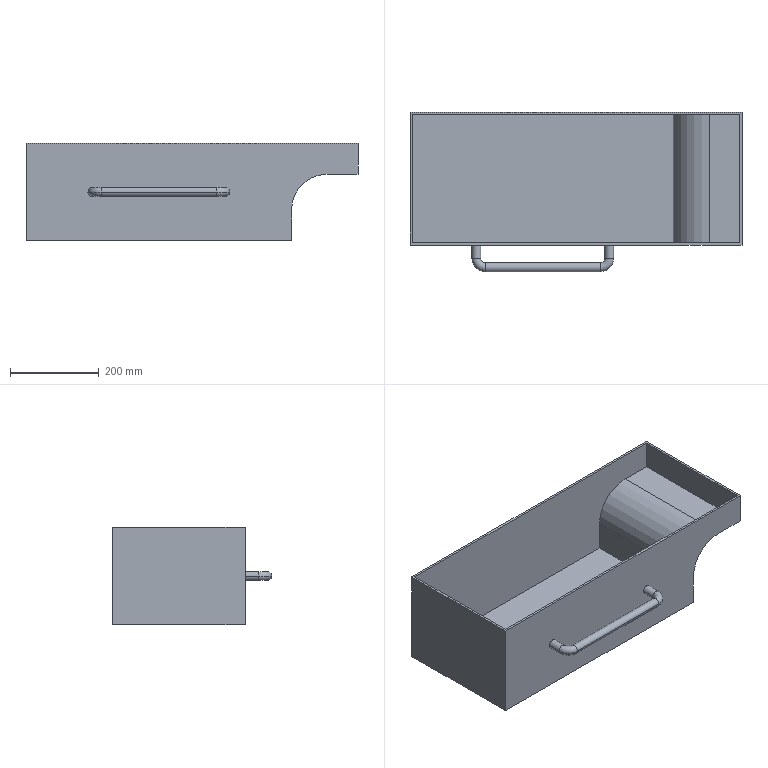Part | STEP file | Sugarcane segment collection box | 1 solid | 27 faces | box 750 x 360 x 220 mm | volume 3249841 mm3 | plane 15 | cylinder 8 | torus 4 | commonest cylinder face diameters 20 x6 160 x1 164 x1
STEP:
#1=CARTESIAN_POINT('',(-130.,-190.,0.));
#2=VERTEX_POINT('',#1);
#3=CARTESIAN_POINT('',(-130.,-210.,0.));
#4=VERTEX_POINT('',#3);
#5=CARTESIAN_POINT('',(-130.,-200.,0.));
#6=DIRECTION('',(-1.,0.,0.));
#7=DIRECTION('',(0.,0.,-1.));
#8=AXIS2_PLACEMENT_3D('',#5,#6,#7);
#9=CIRCLE('',#8,10.);
#10=EDGE_CURVE('',#2,#4,#9,.T.);
#11=ORIENTED_EDGE('',*,*,#10,.T.);
#12=CARTESIAN_POINT('',(-160.,-180.,0.));
#13=VERTEX_POINT('',#12);
#14=CARTESIAN_POINT('',(-130.,-180.,0.));
#15=DIRECTION('',(0.,0.,-1.));
#16=DIRECTION('',(-1.,0.,0.));
#17=AXIS2_PLACEMENT_3D('',#14,#15,#16);
#18=CIRCLE('',#17,30.);
#19=EDGE_CURVE('',#4,#13,#18,.T.);
#20=ORIENTED_EDGE('',*,*,#19,.T.);
#21=CARTESIAN_POINT('',(-140.,-180.,0.));
#22=VERTEX_POINT('',#21);
#23=CARTESIAN_POINT('',(-150.,-180.,0.));
#24=DIRECTION('',(0.,1.,0.));
#25=DIRECTION('',(0.,0.,-1.));
#26=AXIS2_PLACEMENT_3D('',#23,#24,#25);
#27=CIRCLE('',#26,10.);
#28=EDGE_CURVE('',#22,#13,#27,.T.);
#29=ORIENTED_EDGE('',*,*,#28,.F.);
#30=CARTESIAN_POINT('',(-130.,-180.,0.));
#31=DIRECTION('',(0.,0.,-1.));
#32=DIRECTION('',(-1.,0.,0.));
#33=AXIS2_PLACEMENT_3D('',#30,#31,#32);
#34=CIRCLE('',#33,10.);
#35=EDGE_CURVE('',#2,#22,#34,.T.);
#36=ORIENTED_EDGE('',*,*,#35,.F.);
#37=EDGE_LOOP('',(#11,#20,#29,#36));
#38=FACE_OUTER_BOUND('',#37,.T.);
#39=CARTESIAN_POINT('',(-130.,-180.,0.));
#40=DIRECTION('',(0.,0.,-1.));
#41=DIRECTION('',(-1.,0.,0.));
#42=AXIS2_PLACEMENT_3D('',#39,#40,#41);
#43=TOROIDAL_SURFACE('',#42,20.,10.);
#44=ADVANCED_FACE('',(#38),#43,.T.);
#45=CARTESIAN_POINT('',(140.,-180.,0.));
#46=VERTEX_POINT('',#45);
#47=CARTESIAN_POINT('',(160.,-180.,0.));
#48=VERTEX_POINT('',#47);
#49=CARTESIAN_POINT('',(150.,-180.,0.));
#50=DIRECTION('',(0.,-1.,0.));
#51=DIRECTION('',(0.,0.,-1.));
#52=AXIS2_PLACEMENT_3D('',#49,#50,#51);
#53=CIRCLE('',#52,10.);
#54=EDGE_CURVE('',#46,#48,#53,.T.);
#55=ORIENTED_EDGE('',*,*,#54,.T.);
#56=CARTESIAN_POINT('',(130.,-210.,0.));
#57=VERTEX_POINT('',#56);
#58=CARTESIAN_POINT('',(130.,-180.,0.));
#59=DIRECTION('',(0.,0.,-1.));
#60=DIRECTION('',(-1.,0.,0.));
#61=AXIS2_PLACEMENT_3D('',#58,#59,#60);
#62=CIRCLE('',#61,30.);
#63=EDGE_CURVE('',#48,#57,#62,.T.);
#64=ORIENTED_EDGE('',*,*,#63,.T.);
#65=CARTESIAN_POINT('',(130.,-190.,0.));
#66=VERTEX_POINT('',#65);
#67=CARTESIAN_POINT('',(130.,-200.,0.));
#68=DIRECTION('',(-1.,0.,0.));
#69=DIRECTION('',(0.,0.,-1.));
#70=AXIS2_PLACEMENT_3D('',#67,#68,#69);
#71=CIRCLE('',#70,10.);
#72=EDGE_CURVE('',#66,#57,#71,.T.);
#73=ORIENTED_EDGE('',*,*,#72,.F.);
#74=CARTESIAN_POINT('',(130.,-180.,0.));
#75=DIRECTION('',(0.,0.,-1.));
#76=DIRECTION('',(-1.,0.,0.));
#77=AXIS2_PLACEMENT_3D('',#74,#75,#76);
#78=CIRCLE('',#77,10.);
#79=EDGE_CURVE('',#46,#66,#78,.T.);
#80=ORIENTED_EDGE('',*,*,#79,.F.);
#81=EDGE_LOOP('',(#55,#64,#73,#80));
#82=FACE_OUTER_BOUND('',#81,.T.);
#83=CARTESIAN_POINT('',(130.,-180.,0.));
#84=DIRECTION('',(0.,0.,-1.));
#85=DIRECTION('',(-1.,0.,0.));
#86=AXIS2_PLACEMENT_3D('',#83,#84,#85);
#87=TOROIDAL_SURFACE('',#86,20.,10.);
#88=ADVANCED_FACE('',(#82),#87,.T.);
#89=CARTESIAN_POINT('',(-150.,-180.,0.));
#90=DIRECTION('',(0.,1.,0.));
#91=DIRECTION('',(0.,0.,-1.));
#92=AXIS2_PLACEMENT_3D('',#89,#90,#91);
#93=CIRCLE('',#92,10.);
#94=EDGE_CURVE('',#13,#22,#93,.T.);
#95=ORIENTED_EDGE('',*,*,#94,.T.);
#96=CARTESIAN_POINT('',(-140.,-150.,0.));
#97=VERTEX_POINT('',#96);
#98=CARTESIAN_POINT('',(-140.,-180.,0.));
#99=DIRECTION('',(0.,1.,0.));
#100=VECTOR('',#99,1000.);
#101=LINE('',#98,#100);
#102=EDGE_CURVE('',#22,#97,#101,.T.);
#103=ORIENTED_EDGE('',*,*,#102,.T.);
#104=CARTESIAN_POINT('',(-160.,-150.,0.));
#105=VERTEX_POINT('',#104);
#106=CARTESIAN_POINT('',(-150.,-150.,0.));
#107=DIRECTION('',(0.,1.,0.));
#108=DIRECTION('',(0.,0.,-1.));
#109=AXIS2_PLACEMENT_3D('',#106,#107,#108);
#110=CIRCLE('',#109,10.);
#111=EDGE_CURVE('',#105,#97,#110,.T.);
#112=ORIENTED_EDGE('',*,*,#111,.F.);
#113=CARTESIAN_POINT('',(-160.,-180.,0.));
#114=DIRECTION('',(0.,1.,0.));
#115=VECTOR('',#114,1000.);
#116=LINE('',#113,#115);
#117=EDGE_CURVE('',#13,#105,#116,.T.);
#118=ORIENTED_EDGE('',*,*,#117,.F.);
#119=EDGE_LOOP('',(#95,#103,#112,#118));
#120=FACE_OUTER_BOUND('',#119,.T.);
#121=CARTESIAN_POINT('',(-150.,-180.,0.));
#122=DIRECTION('',(0.,1.,0.));
#123=DIRECTION('',(-1.,0.,0.));
#124=AXIS2_PLACEMENT_3D('',#121,#122,#123);
#125=CYLINDRICAL_SURFACE('',#124,10.);
#126=ADVANCED_FACE('',(#120),#125,.T.);
#127=CARTESIAN_POINT('',(130.,-200.,0.));
#128=DIRECTION('',(-1.,0.,0.));
#129=DIRECTION('',(0.,0.,-1.));
#130=AXIS2_PLACEMENT_3D('',#127,#128,#129);
#131=CIRCLE('',#130,10.);
#132=EDGE_CURVE('',#57,#66,#131,.T.);
#133=ORIENTED_EDGE('',*,*,#132,.T.);
#134=CARTESIAN_POINT('',(130.,-190.,0.));
#135=DIRECTION('',(-1.,0.,0.));
#136=VECTOR('',#135,1000.);
#137=LINE('',#134,#136);
#138=EDGE_CURVE('',#66,#2,#137,.T.);
#139=ORIENTED_EDGE('',*,*,#138,.T.);
#140=CARTESIAN_POINT('',(-130.,-200.,0.));
#141=DIRECTION('',(-1.,0.,0.));
#142=DIRECTION('',(0.,0.,-1.));
#143=AXIS2_PLACEMENT_3D('',#140,#141,#142);
#144=CIRCLE('',#143,10.);
#145=EDGE_CURVE('',#4,#2,#144,.T.);
#146=ORIENTED_EDGE('',*,*,#145,.F.);
#147=CARTESIAN_POINT('',(130.,-210.,0.));
#148=DIRECTION('',(-1.,0.,0.));
#149=VECTOR('',#148,1000.);
#150=LINE('',#147,#149);
#151=EDGE_CURVE('',#57,#4,#150,.T.);
#152=ORIENTED_EDGE('',*,*,#151,.F.);
#153=EDGE_LOOP('',(#133,#139,#146,#152));
#154=FACE_OUTER_BOUND('',#153,.T.);
#155=CARTESIAN_POINT('',(130.,-200.,0.));
#156=DIRECTION('',(-1.,0.,0.));
#157=DIRECTION('',(0.,-1.,0.));
#158=AXIS2_PLACEMENT_3D('',#155,#156,#157);
#159=CYLINDRICAL_SURFACE('',#158,10.);
#160=ADVANCED_FACE('',(#154),#159,.T.);
#161=CARTESIAN_POINT('',(160.,-150.,0.));
#162=VERTEX_POINT('',#161);
#163=CARTESIAN_POINT('',(140.,-150.,0.));
#164=VERTEX_POINT('',#163);
#165=CARTESIAN_POINT('',(150.,-150.,0.));
#166=DIRECTION('',(0.,-1.,0.));
#167=DIRECTION('',(0.,0.,-1.));
#168=AXIS2_PLACEMENT_3D('',#165,#166,#167);
#169=CIRCLE('',#168,10.);
#170=EDGE_CURVE('',#162,#164,#169,.T.);
#171=ORIENTED_EDGE('',*,*,#170,.T.);
#172=CARTESIAN_POINT('',(140.,-150.,0.));
#173=DIRECTION('',(0.,-1.,0.));
#174=VECTOR('',#173,1000.);
#175=LINE('',#172,#174);
#176=EDGE_CURVE('',#164,#46,#175,.T.);
#177=ORIENTED_EDGE('',*,*,#176,.T.);
#178=CARTESIAN_POINT('',(150.,-180.,0.));
#179=DIRECTION('',(0.,-1.,0.));
#180=DIRECTION('',(0.,0.,-1.));
#181=AXIS2_PLACEMENT_3D('',#178,#179,#180);
#182=CIRCLE('',#181,10.);
#183=EDGE_CURVE('',#48,#46,#182,.T.);
#184=ORIENTED_EDGE('',*,*,#183,.F.);
#185=CARTESIAN_POINT('',(160.,-150.,0.));
#186=DIRECTION('',(0.,-1.,0.));
#187=VECTOR('',#186,1000.);
#188=LINE('',#185,#187);
#189=EDGE_CURVE('',#162,#48,#188,.T.);
#190=ORIENTED_EDGE('',*,*,#189,.F.);
#191=EDGE_LOOP('',(#171,#177,#184,#190));
#192=FACE_OUTER_BOUND('',#191,.T.);
#193=CARTESIAN_POINT('',(150.,-150.,0.));
#194=DIRECTION('',(0.,-1.,0.));
#195=DIRECTION('',(1.,0.,0.));
#196=AXIS2_PLACEMENT_3D('',#193,#194,#195);
#197=CYLINDRICAL_SURFACE('',#196,10.);
#198=ADVANCED_FACE('',(#192),#197,.T.);
#199=CARTESIAN_POINT('',(445.,145.,110.));
#200=VERTEX_POINT('',#199);
#201=CARTESIAN_POINT('',(445.,-145.,110.));
#202=VERTEX_POINT('',#201);
#203=CARTESIAN_POINT('',(445.,0.,110.));
#204=DIRECTION('',(0.,-1.,0.));
#205=VECTOR('',#204,1000.);
#206=LINE('',#203,#205);
#207=EDGE_CURVE('',#200,#202,#206,.T.);
#208=ORIENTED_EDGE('',*,*,#207,.T.);
#209=CARTESIAN_POINT('',(-295.,-145.,110.));
#210=VERTEX_POINT('',#209);
#211=CARTESIAN_POINT('',(-300.,-145.,110.));
#212=DIRECTION('',(1.,0.,0.));
#213=VECTOR('',#212,1000.);
#214=LINE('',#211,#213);
#215=EDGE_CURVE('',#210,#202,#214,.T.);
#216=ORIENTED_EDGE('',*,*,#215,.F.);
#217=CARTESIAN_POINT('',(-295.,145.,110.));
#218=VERTEX_POINT('',#217);
#219=CARTESIAN_POINT('',(-295.,150.,110.));
#220=DIRECTION('',(0.,-1.,0.));
#221=VECTOR('',#220,1000.);
#222=LINE('',#219,#221);
#223=EDGE_CURVE('',#218,#210,#222,.T.);
#224=ORIENTED_EDGE('',*,*,#223,.F.);
#225=CARTESIAN_POINT('',(-300.,145.,110.));
#226=DIRECTION('',(-1.,0.,0.));
#227=VECTOR('',#226,1000.);
#228=LINE('',#225,#227);
#229=EDGE_CURVE('',#200,#218,#228,.T.);
#230=ORIENTED_EDGE('',*,*,#229,.F.);
#231=EDGE_LOOP('',(#208,#216,#224,#230));
#232=FACE_BOUND('',#231,.T.);
#233=CARTESIAN_POINT('',(-300.,-150.,110.));
#234=VERTEX_POINT('',#233);
#235=CARTESIAN_POINT('',(450.,-150.,110.));
#236=VERTEX_POINT('',#235);
#237=CARTESIAN_POINT('',(-300.,-150.,110.));
#238=DIRECTION('',(1.,0.,0.));
#239=VECTOR('',#238,1000.);
#240=LINE('',#237,#239);
#241=EDGE_CURVE('',#234,#236,#240,.T.);
#242=ORIENTED_EDGE('',*,*,#241,.T.);
#243=CARTESIAN_POINT('',(450.,150.,110.));
#244=VERTEX_POINT('',#243);
#245=CARTESIAN_POINT('',(450.,-150.,110.));
#246=DIRECTION('',(0.,-1.,0.));
#247=VECTOR('',#246,1000.);
#248=LINE('',#245,#247);
#249=EDGE_CURVE('',#244,#236,#248,.T.);
#250=ORIENTED_EDGE('',*,*,#249,.F.);
#251=CARTESIAN_POINT('',(-300.,150.,110.));
#252=VERTEX_POINT('',#251);
#253=CARTESIAN_POINT('',(-300.,150.,110.));
#254=DIRECTION('',(-1.,0.,0.));
#255=VECTOR('',#254,1000.);
#256=LINE('',#253,#255);
#257=EDGE_CURVE('',#244,#252,#256,.T.);
#258=ORIENTED_EDGE('',*,*,#257,.T.);
#259=CARTESIAN_POINT('',(-300.,150.,110.));
#260=DIRECTION('',(0.,-1.,0.));
#261=VECTOR('',#260,1000.);
#262=LINE('',#259,#261);
#263=EDGE_CURVE('',#252,#234,#262,.T.);
#264=ORIENTED_EDGE('',*,*,#263,.T.);
#265=EDGE_LOOP('',(#242,#250,#258,#264));
#266=FACE_OUTER_BOUND('',#265,.T.);
#267=CARTESIAN_POINT('',(0.,0.,110.));
#268=DIRECTION('',(0.,0.,1.));
#269=DIRECTION('',(1.,0.,0.));
#270=AXIS2_PLACEMENT_3D('',#267,#268,#269);
#271=PLANE('',#270);
#272=ADVANCED_FACE('',(#232,#266),#271,.T.);
#273=CARTESIAN_POINT('',(300.,150.,-40.));
#274=VERTEX_POINT('',#273);
#275=CARTESIAN_POINT('',(300.,150.,-110.));
#276=VERTEX_POINT('',#275);
#277=CARTESIAN_POINT('',(300.,150.,110.));
#278=DIRECTION('',(0.,0.,-1.));
#279=VECTOR('',#278,1000.);
#280=LINE('',#277,#279);
#281=EDGE_CURVE('',#274,#276,#280,.T.);
#282=ORIENTED_EDGE('',*,*,#281,.F.);
#283=CARTESIAN_POINT('',(300.,-150.,-40.));
#284=VERTEX_POINT('',#283);
#285=CARTESIAN_POINT('',(300.,-150.,-40.));
#286=DIRECTION('',(0.,-1.,0.));
#287=VECTOR('',#286,1000.);
#288=LINE('',#285,#287);
#289=EDGE_CURVE('',#274,#284,#288,.T.);
#290=ORIENTED_EDGE('',*,*,#289,.T.);
#291=CARTESIAN_POINT('',(300.,-150.,-110.));
#292=VERTEX_POINT('',#291);
#293=CARTESIAN_POINT('',(300.,-150.,110.));
#294=DIRECTION('',(0.,0.,-1.));
#295=VECTOR('',#294,1000.);
#296=LINE('',#293,#295);
#297=EDGE_CURVE('',#284,#292,#296,.T.);
#298=ORIENTED_EDGE('',*,*,#297,.T.);
#299=CARTESIAN_POINT('',(300.,150.,-110.));
#300=DIRECTION('',(0.,1.,0.));
#301=VECTOR('',#300,1000.);
#302=LINE('',#299,#301);
#303=EDGE_CURVE('',#292,#276,#302,.T.);
#304=ORIENTED_EDGE('',*,*,#303,.T.);
#305=EDGE_LOOP('',(#282,#290,#298,#304));
#306=FACE_OUTER_BOUND('',#305,.T.);
#307=CARTESIAN_POINT('',(300.,150.,110.));
#308=DIRECTION('',(-1.,0.,0.));
#309=DIRECTION('',(0.,0.,1.));
#310=AXIS2_PLACEMENT_3D('',#307,#308,#309);
#311=PLANE('',#310);
#312=ADVANCED_FACE('',(#306),#311,.F.);
#313=ORIENTED_EDGE('',*,*,#170,.F.);
#314=CARTESIAN_POINT('',(150.,-150.,0.));
#315=DIRECTION('',(0.,-1.,0.));
#316=DIRECTION('',(0.,0.,-1.));
#317=AXIS2_PLACEMENT_3D('',#314,#315,#316);
#318=CIRCLE('',#317,10.);
#319=EDGE_CURVE('',#164,#162,#318,.T.);
#320=ORIENTED_EDGE('',*,*,#319,.F.);
#321=EDGE_LOOP('',(#313,#320));
#322=FACE_BOUND('',#321,.T.);
#323=CARTESIAN_POINT('',(-300.,-150.,-110.));
#324=VERTEX_POINT('',#323);
#325=CARTESIAN_POINT('',(-300.,-150.,-110.));
#326=DIRECTION('',(1.,0.,0.));
#327=VECTOR('',#326,1000.);
#328=LINE('',#325,#327);
#329=EDGE_CURVE('',#324,#292,#328,.T.);
#330=ORIENTED_EDGE('',*,*,#329,.T.);
#331=ORIENTED_EDGE('',*,*,#297,.F.);
#332=CARTESIAN_POINT('',(380.,-150.,40.));
#333=VERTEX_POINT('',#332);
#334=CARTESIAN_POINT('',(380.,-150.,-40.));
#335=DIRECTION('',(0.,1.,0.));
#336=DIRECTION('',(0.,0.,1.));
#337=AXIS2_PLACEMENT_3D('',#334,#335,#336);
#338=CIRCLE('',#337,80.);
#339=EDGE_CURVE('',#284,#333,#338,.T.);
#340=ORIENTED_EDGE('',*,*,#339,.T.);
#341=CARTESIAN_POINT('',(450.,-150.,40.));
#342=VERTEX_POINT('',#341);
#343=CARTESIAN_POINT('',(450.,-150.,40.));
#344=DIRECTION('',(-1.,0.,0.));
#345=VECTOR('',#344,1000.);
#346=LINE('',#343,#345);
#347=EDGE_CURVE('',#342,#333,#346,.T.);
#348=ORIENTED_EDGE('',*,*,#347,.F.);
#349=CARTESIAN_POINT('',(450.,-150.,110.));
#350=DIRECTION('',(0.,0.,-1.));
#351=VECTOR('',#350,1000.);
#352=LINE('',#349,#351);
#353=EDGE_CURVE('',#236,#342,#352,.T.);
#354=ORIENTED_EDGE('',*,*,#353,.F.);
#355=ORIENTED_EDGE('',*,*,#241,.F.);
#356=CARTESIAN_POINT('',(-300.,-150.,110.));
#357=DIRECTION('',(0.,0.,-1.));
#358=VECTOR('',#357,1000.);
#359=LINE('',#356,#358);
#360=EDGE_CURVE('',#234,#324,#359,.T.);
#361=ORIENTED_EDGE('',*,*,#360,.T.);
#362=EDGE_LOOP('',(#330,#331,#340,#348,#354,#355,#361));
#363=FACE_OUTER_BOUND('',#362,.T.);
#364=ORIENTED_EDGE('',*,*,#111,.T.);
#365=CARTESIAN_POINT('',(-150.,-150.,0.));
#366=DIRECTION('',(0.,1.,0.));
#367=DIRECTION('',(0.,0.,-1.));
#368=AXIS2_PLACEMENT_3D('',#365,#366,#367);
#369=CIRCLE('',#368,10.);
#370=EDGE_CURVE('',#97,#105,#369,.T.);
#371=ORIENTED_EDGE('',*,*,#370,.T.);
#372=EDGE_LOOP('',(#364,#371));
#373=FACE_BOUND('',#372,.T.);
#374=CARTESIAN_POINT('',(-300.,-150.,110.));
#375=DIRECTION('',(0.,1.,0.));
#376=DIRECTION('',(0.,0.,1.));
#377=AXIS2_PLACEMENT_3D('',#374,#375,#376);
#378=PLANE('',#377);
#379=ADVANCED_FACE('',(#322,#363,#373),#378,.F.);
#380=CARTESIAN_POINT('',(-300.,150.,-110.));
#381=VERTEX_POINT('',#380);
#382=CARTESIAN_POINT('',(-300.,150.,-110.));
#383=DIRECTION('',(-1.,0.,0.));
#384=VECTOR('',#383,1000.);
#385=LINE('',#382,#384);
#386=EDGE_CURVE('',#276,#381,#385,.T.);
#387=ORIENTED_EDGE('',*,*,#386,.T.);
#388=CARTESIAN_POINT('',(-300.,150.,110.));
#389=DIRECTION('',(0.,0.,-1.));
#390=VECTOR('',#389,1000.);
#391=LINE('',#388,#390);
#392=EDGE_CURVE('',#252,#381,#391,.T.);
#393=ORIENTED_EDGE('',*,*,#392,.F.);
#394=ORIENTED_EDGE('',*,*,#257,.F.);
#395=CARTESIAN_POINT('',(450.,150.,40.));
#396=VERTEX_POINT('',#395);
#397=CARTESIAN_POINT('',(450.,150.,110.));
#398=DIRECTION('',(0.,0.,1.));
#399=VECTOR('',#398,1000.);
#400=LINE('',#397,#399);
#401=EDGE_CURVE('',#396,#244,#400,.T.);
#402=ORIENTED_EDGE('',*,*,#401,.F.);
#403=CARTESIAN_POINT('',(380.,150.,40.));
#404=VERTEX_POINT('',#403);
#405=CARTESIAN_POINT('',(450.,150.,40.));
#406=DIRECTION('',(-1.,0.,0.));
#407=VECTOR('',#406,1000.);
#408=LINE('',#405,#407);
#409=EDGE_CURVE('',#396,#404,#408,.T.);
#410=ORIENTED_EDGE('',*,*,#409,.T.);
#411=CARTESIAN_POINT('',(380.,150.,-40.));
#412=DIRECTION('',(0.,-1.,0.));
#413=DIRECTION('',(0.,0.,-1.));
#414=AXIS2_PLACEMENT_3D('',#411,#412,#413);
#415=CIRCLE('',#414,80.);
#416=EDGE_CURVE('',#404,#274,#415,.T.);
#417=ORIENTED_EDGE('',*,*,#416,.T.);
#418=ORIENTED_EDGE('',*,*,#281,.T.);
#419=EDGE_LOOP('',(#387,#393,#394,#402,#410,#417,#418));
#420=FACE_OUTER_BOUND('',#419,.T.);
#421=CARTESIAN_POINT('',(-300.,150.,110.));
#422=DIRECTION('',(0.,-1.,0.));
#423=DIRECTION('',(0.,0.,-1.));
#424=AXIS2_PLACEMENT_3D('',#421,#422,#423);
#425=PLANE('',#424);
#426=ADVANCED_FACE('',(#420),#425,.F.);
#427=CARTESIAN_POINT('',(-300.,150.,-110.));
#428=DIRECTION('',(0.,-1.,0.));
#429=VECTOR('',#428,1000.);
#430=LINE('',#427,#429);
#431=EDGE_CURVE('',#381,#324,#430,.T.);
#432=ORIENTED_EDGE('',*,*,#431,.T.);
#433=ORIENTED_EDGE('',*,*,#360,.F.);
#434=ORIENTED_EDGE('',*,*,#263,.F.);
#435=ORIENTED_EDGE('',*,*,#392,.T.);
#436=EDGE_LOOP('',(#432,#433,#434,#435));
#437=FACE_OUTER_BOUND('',#436,.T.);
#438=CARTESIAN_POINT('',(-300.,150.,110.));
#439=DIRECTION('',(1.,0.,0.));
#440=DIRECTION('',(0.,0.,-1.));
#441=AXIS2_PLACEMENT_3D('',#438,#439,#440);
#442=PLANE('',#441);
#443=ADVANCED_FACE('',(#437),#442,.F.);
#444=ORIENTED_EDGE('',*,*,#303,.F.);
#445=ORIENTED_EDGE('',*,*,#329,.F.);
#446=ORIENTED_EDGE('',*,*,#431,.F.);
#447=ORIENTED_EDGE('',*,*,#386,.F.);
#448=EDGE_LOOP('',(#444,#445,#446,#447));
#449=FACE_OUTER_BOUND('',#448,.T.);
#450=CARTESIAN_POINT('',(0.,0.,-110.));
#451=DIRECTION('',(0.,0.,1.));
#452=DIRECTION('',(1.,0.,0.));
#453=AXIS2_PLACEMENT_3D('',#450,#451,#452);
#454=PLANE('',#453);
#455=ADVANCED_FACE('',(#449),#454,.F.);
#456=CARTESIAN_POINT('',(295.,-145.,-37.));
#457=VERTEX_POINT('',#456);
#458=CARTESIAN_POINT('',(295.,-145.,-105.));
#459=VERTEX_POINT('',#458);
#460=CARTESIAN_POINT('',(295.,-145.,110.));
#461=DIRECTION('',(0.,0.,-1.));
#462=VECTOR('',#461,1000.);
#463=LINE('',#460,#462);
#464=EDGE_CURVE('',#457,#459,#463,.T.);
#465=ORIENTED_EDGE('',*,*,#464,.F.);
#466=CARTESIAN_POINT('',(295.,145.,-37.));
#467=VERTEX_POINT('',#466);
#468=CARTESIAN_POINT('',(295.,150.,-37.));
#469=DIRECTION('',(0.,1.,0.));
#470=VECTOR('',#469,1000.);
#471=LINE('',#468,#470);
#472=EDGE_CURVE('',#457,#467,#471,.T.);
#473=ORIENTED_EDGE('',*,*,#472,.T.);
#474=CARTESIAN_POINT('',(295.,145.,-105.));
#475=VERTEX_POINT('',#474);
#476=CARTESIAN_POINT('',(295.,145.,110.));
#477=DIRECTION('',(0.,0.,-1.));
#478=VECTOR('',#477,1000.);
#479=LINE('',#476,#478);
#480=EDGE_CURVE('',#467,#475,#479,.T.);
#481=ORIENTED_EDGE('',*,*,#480,.T.);
#482=CARTESIAN_POINT('',(295.,150.,-105.));
#483=DIRECTION('',(0.,1.,0.));
#484=VECTOR('',#483,1000.);
#485=LINE('',#482,#484);
#486=EDGE_CURVE('',#459,#475,#485,.T.);
#487=ORIENTED_EDGE('',*,*,#486,.F.);
#488=EDGE_LOOP('',(#465,#473,#481,#487));
#489=FACE_OUTER_BOUND('',#488,.T.);
#490=CARTESIAN_POINT('',(295.,150.,110.));
#491=DIRECTION('',(-1.,0.,0.));
#492=DIRECTION('',(0.,0.,1.));
#493=AXIS2_PLACEMENT_3D('',#490,#491,#492);
#494=PLANE('',#493);
#495=ADVANCED_FACE('',(#489),#494,.T.);
#496=ORIENTED_EDGE('',*,*,#480,.F.);
#497=CARTESIAN_POINT('',(377.,145.,45.));
#498=VERTEX_POINT('',#497);
#499=CARTESIAN_POINT('',(377.,145.,-37.));
#500=DIRECTION('',(0.,1.,0.));
#501=DIRECTION('',(0.,0.,-1.));
#502=AXIS2_PLACEMENT_3D('',#499,#500,#501);
#503=CIRCLE('',#502,82.);
#504=EDGE_CURVE('',#467,#498,#503,.T.);
#505=ORIENTED_EDGE('',*,*,#504,.T.);
#506=CARTESIAN_POINT('',(445.,145.,45.));
#507=VERTEX_POINT('',#506);
#508=CARTESIAN_POINT('',(-300.,145.,45.));
#509=DIRECTION('',(-1.,0.,0.));
#510=VECTOR('',#509,1000.);
#511=LINE('',#508,#510);
#512=EDGE_CURVE('',#507,#498,#511,.T.);
#513=ORIENTED_EDGE('',*,*,#512,.F.);
#514=CARTESIAN_POINT('',(445.,145.,0.));
#515=DIRECTION('',(0.,0.,1.));
#516=VECTOR('',#515,1000.);
#517=LINE('',#514,#516);
#518=EDGE_CURVE('',#507,#200,#517,.T.);
#519=ORIENTED_EDGE('',*,*,#518,.T.);
#520=ORIENTED_EDGE('',*,*,#229,.T.);
#521=CARTESIAN_POINT('',(-295.,145.,-105.));
#522=VERTEX_POINT('',#521);
#523=CARTESIAN_POINT('',(-295.,145.,110.));
#524=DIRECTION('',(0.,0.,-1.));
#525=VECTOR('',#524,1000.);
#526=LINE('',#523,#525);
#527=EDGE_CURVE('',#218,#522,#526,.T.);
#528=ORIENTED_EDGE('',*,*,#527,.T.);
#529=CARTESIAN_POINT('',(-300.,145.,-105.));
#530=DIRECTION('',(-1.,0.,0.));
#531=VECTOR('',#530,1000.);
#532=LINE('',#529,#531);
#533=EDGE_CURVE('',#475,#522,#532,.T.);
#534=ORIENTED_EDGE('',*,*,#533,.F.);
#535=EDGE_LOOP('',(#496,#505,#513,#519,#520,#528,#534));
#536=FACE_OUTER_BOUND('',#535,.T.);
#537=CARTESIAN_POINT('',(-300.,145.,110.));
#538=DIRECTION('',(0.,-1.,0.));
#539=DIRECTION('',(0.,0.,-1.));
#540=AXIS2_PLACEMENT_3D('',#537,#538,#539);
#541=PLANE('',#540);
#542=ADVANCED_FACE('',(#536),#541,.T.);
#543=CARTESIAN_POINT('',(-295.,-145.,-105.));
#544=VERTEX_POINT('',#543);
#545=CARTESIAN_POINT('',(-295.,150.,-105.));
#546=DIRECTION('',(0.,-1.,0.));
#547=VECTOR('',#546,1000.);
#548=LINE('',#545,#547);
#549=EDGE_CURVE('',#522,#544,#548,.T.);
#550=ORIENTED_EDGE('',*,*,#549,.F.);
#551=ORIENTED_EDGE('',*,*,#527,.F.);
#552=ORIENTED_EDGE('',*,*,#223,.T.);
#553=CARTESIAN_POINT('',(-295.,-145.,110.));
#554=DIRECTION('',(0.,0.,-1.));
#555=VECTOR('',#554,1000.);
#556=LINE('',#553,#555);
#557=EDGE_CURVE('',#210,#544,#556,.T.);
#558=ORIENTED_EDGE('',*,*,#557,.T.);
#559=EDGE_LOOP('',(#550,#551,#552,#558));
#560=FACE_OUTER_BOUND('',#559,.T.);
#561=CARTESIAN_POINT('',(-295.,150.,110.));
#562=DIRECTION('',(1.,0.,0.));
#563=DIRECTION('',(0.,0.,-1.));
#564=AXIS2_PLACEMENT_3D('',#561,#562,#563);
#565=PLANE('',#564);
#566=ADVANCED_FACE('',(#560),#565,.T.);
#567=ORIENTED_EDGE('',*,*,#215,.T.);
#568=CARTESIAN_POINT('',(445.,-145.,45.));
#569=VERTEX_POINT('',#568);
#570=CARTESIAN_POINT('',(445.,-145.,0.));
#571=DIRECTION('',(0.,0.,-1.));
#572=VECTOR('',#571,1000.);
#573=LINE('',#570,#572);
#574=EDGE_CURVE('',#202,#569,#573,.T.);
#575=ORIENTED_EDGE('',*,*,#574,.T.);
#576=CARTESIAN_POINT('',(377.,-145.,45.));
#577=VERTEX_POINT('',#576);
#578=CARTESIAN_POINT('',(450.,-145.,45.));
#579=DIRECTION('',(-1.,0.,0.));
#580=VECTOR('',#579,1000.);
#581=LINE('',#578,#580);
#582=EDGE_CURVE('',#569,#577,#581,.T.);
#583=ORIENTED_EDGE('',*,*,#582,.T.);
#584=CARTESIAN_POINT('',(377.,-145.,-37.));
#585=DIRECTION('',(0.,-1.,0.));
#586=DIRECTION('',(0.,0.,1.));
#587=AXIS2_PLACEMENT_3D('',#584,#585,#586);
#588=CIRCLE('',#587,82.);
#589=EDGE_CURVE('',#577,#457,#588,.T.);
#590=ORIENTED_EDGE('',*,*,#589,.T.);
#591=ORIENTED_EDGE('',*,*,#464,.T.);
#592=CARTESIAN_POINT('',(-300.,-145.,-105.));
#593=DIRECTION('',(1.,0.,0.));
#594=VECTOR('',#593,1000.);
#595=LINE('',#592,#594);
#596=EDGE_CURVE('',#544,#459,#595,.T.);
#597=ORIENTED_EDGE('',*,*,#596,.F.);
#598=ORIENTED_EDGE('',*,*,#557,.F.);
#599=EDGE_LOOP('',(#567,#575,#583,#590,#591,#597,#598));
#600=FACE_OUTER_BOUND('',#599,.T.);
#601=CARTESIAN_POINT('',(-300.,-145.,110.));
#602=DIRECTION('',(0.,1.,0.));
#603=DIRECTION('',(0.,0.,1.));
#604=AXIS2_PLACEMENT_3D('',#601,#602,#603);
#605=PLANE('',#604);
#606=ADVANCED_FACE('',(#600),#605,.T.);
#607=ORIENTED_EDGE('',*,*,#486,.T.);
#608=ORIENTED_EDGE('',*,*,#533,.T.);
#609=ORIENTED_EDGE('',*,*,#549,.T.);
#610=ORIENTED_EDGE('',*,*,#596,.T.);
#611=EDGE_LOOP('',(#607,#608,#609,#610));
#612=FACE_OUTER_BOUND('',#611,.T.);
#613=CARTESIAN_POINT('',(0.,0.,-105.));
#614=DIRECTION('',(0.,0.,1.));
#615=DIRECTION('',(1.,0.,0.));
#616=AXIS2_PLACEMENT_3D('',#613,#614,#615);
#617=PLANE('',#616);
#618=ADVANCED_FACE('',(#612),#617,.T.);
#619=ORIENTED_EDGE('',*,*,#102,.F.);
#620=ORIENTED_EDGE('',*,*,#28,.T.);
#621=ORIENTED_EDGE('',*,*,#117,.T.);
#622=ORIENTED_EDGE('',*,*,#370,.F.);
#623=EDGE_LOOP('',(#619,#620,#621,#622));
#624=FACE_OUTER_BOUND('',#623,.T.);
#625=CARTESIAN_POINT('',(-150.,-180.,0.));
#626=DIRECTION('',(0.,1.,0.));
#627=DIRECTION('',(-1.,0.,0.));
#628=AXIS2_PLACEMENT_3D('',#625,#626,#627);
#629=CYLINDRICAL_SURFACE('',#628,10.);
#630=ADVANCED_FACE('',(#624),#629,.T.);
#631=ORIENTED_EDGE('',*,*,#19,.F.);
#632=ORIENTED_EDGE('',*,*,#145,.T.);
#633=ORIENTED_EDGE('',*,*,#35,.T.);
#634=ORIENTED_EDGE('',*,*,#94,.F.);
#635=EDGE_LOOP('',(#631,#632,#633,#634));
#636=FACE_OUTER_BOUND('',#635,.T.);
#637=CARTESIAN_POINT('',(-130.,-180.,0.));
#638=DIRECTION('',(0.,0.,-1.));
#639=DIRECTION('',(-1.,0.,0.));
#640=AXIS2_PLACEMENT_3D('',#637,#638,#639);
#641=TOROIDAL_SURFACE('',#640,20.,10.);
#642=ADVANCED_FACE('',(#636),#641,.T.);
#643=ORIENTED_EDGE('',*,*,#138,.F.);
#644=ORIENTED_EDGE('',*,*,#72,.T.);
#645=ORIENTED_EDGE('',*,*,#151,.T.);
#646=ORIENTED_EDGE('',*,*,#10,.F.);
#647=EDGE_LOOP('',(#643,#644,#645,#646));
#648=FACE_OUTER_BOUND('',#647,.T.);
#649=CARTESIAN_POINT('',(130.,-200.,0.));
#650=DIRECTION('',(-1.,0.,0.));
#651=DIRECTION('',(0.,-1.,0.));
#652=AXIS2_PLACEMENT_3D('',#649,#650,#651);
#653=CYLINDRICAL_SURFACE('',#652,10.);
#654=ADVANCED_FACE('',(#648),#653,.T.);
#655=ORIENTED_EDGE('',*,*,#63,.F.);
#656=ORIENTED_EDGE('',*,*,#183,.T.);
#657=ORIENTED_EDGE('',*,*,#79,.T.);
#658=ORIENTED_EDGE('',*,*,#132,.F.);
#659=EDGE_LOOP('',(#655,#656,#657,#658));
#660=FACE_OUTER_BOUND('',#659,.T.);
#661=CARTESIAN_POINT('',(130.,-180.,0.));
#662=DIRECTION('',(0.,0.,-1.));
#663=DIRECTION('',(-1.,0.,0.));
#664=AXIS2_PLACEMENT_3D('',#661,#662,#663);
#665=TOROIDAL_SURFACE('',#664,20.,10.);
#666=ADVANCED_FACE('',(#660),#665,.T.);
#667=ORIENTED_EDGE('',*,*,#176,.F.);
#668=ORIENTED_EDGE('',*,*,#319,.T.);
#669=ORIENTED_EDGE('',*,*,#189,.T.);
#670=ORIENTED_EDGE('',*,*,#54,.F.);
#671=EDGE_LOOP('',(#667,#668,#669,#670));
#672=FACE_OUTER_BOUND('',#671,.T.);
#673=CARTESIAN_POINT('',(150.,-150.,0.));
#674=DIRECTION('',(0.,-1.,0.));
#675=DIRECTION('',(1.,0.,0.));
#676=AXIS2_PLACEMENT_3D('',#673,#674,#675);
#677=CYLINDRICAL_SURFACE('',#676,10.);
#678=ADVANCED_FACE('',(#672),#677,.T.);
#679=ORIENTED_EDGE('',*,*,#347,.T.);
#680=CARTESIAN_POINT('',(380.,150.,40.));
#681=DIRECTION('',(0.,1.,0.));
#682=VECTOR('',#681,1000.);
#683=LINE('',#680,#682);
#684=EDGE_CURVE('',#333,#404,#683,.T.);
#685=ORIENTED_EDGE('',*,*,#684,.T.);
#686=ORIENTED_EDGE('',*,*,#409,.F.);
#687=CARTESIAN_POINT('',(450.,-150.,40.));
#688=DIRECTION('',(0.,1.,0.));
#689=VECTOR('',#688,1000.);
#690=LINE('',#687,#689);
#691=EDGE_CURVE('',#342,#396,#690,.T.);
#692=ORIENTED_EDGE('',*,*,#691,.F.);
#693=EDGE_LOOP('',(#679,#685,#686,#692));
#694=FACE_OUTER_BOUND('',#693,.T.);
#695=CARTESIAN_POINT('',(450.,-150.,40.));
#696=DIRECTION('',(0.,0.,1.));
#697=DIRECTION('',(1.,0.,0.));
#698=AXIS2_PLACEMENT_3D('',#695,#696,#697);
#699=PLANE('',#698);
#700=ADVANCED_FACE('',(#694),#699,.F.);
#701=ORIENTED_EDGE('',*,*,#249,.T.);
#702=ORIENTED_EDGE('',*,*,#353,.T.);
#703=ORIENTED_EDGE('',*,*,#691,.T.);
#704=ORIENTED_EDGE('',*,*,#401,.T.);
#705=EDGE_LOOP('',(#701,#702,#703,#704));
#706=FACE_OUTER_BOUND('',#705,.T.);
#707=CARTESIAN_POINT('',(450.,0.,0.));
#708=DIRECTION('',(-1.,0.,0.));
#709=DIRECTION('',(0.,0.,1.));
#710=AXIS2_PLACEMENT_3D('',#707,#708,#709);
#711=PLANE('',#710);
#712=ADVANCED_FACE('',(#706),#711,.F.);
#713=ORIENTED_EDGE('',*,*,#512,.T.);
#714=CARTESIAN_POINT('',(377.,-150.,45.));
#715=DIRECTION('',(0.,-1.,0.));
#716=VECTOR('',#715,1000.);
#717=LINE('',#714,#716);
#718=EDGE_CURVE('',#498,#577,#717,.T.);
#719=ORIENTED_EDGE('',*,*,#718,.T.);
#720=ORIENTED_EDGE('',*,*,#582,.F.);
#721=CARTESIAN_POINT('',(445.,0.,45.));
#722=DIRECTION('',(0.,1.,0.));
#723=VECTOR('',#722,1000.);
#724=LINE('',#721,#723);
#725=EDGE_CURVE('',#569,#507,#724,.T.);
#726=ORIENTED_EDGE('',*,*,#725,.T.);
#727=EDGE_LOOP('',(#713,#719,#720,#726));
#728=FACE_OUTER_BOUND('',#727,.T.);
#729=CARTESIAN_POINT('',(450.,-150.,45.));
#730=DIRECTION('',(0.,0.,1.));
#731=DIRECTION('',(1.,0.,0.));
#732=AXIS2_PLACEMENT_3D('',#729,#730,#731);
#733=PLANE('',#732);
#734=ADVANCED_FACE('',(#728),#733,.T.);
#735=ORIENTED_EDGE('',*,*,#207,.F.);
#736=ORIENTED_EDGE('',*,*,#518,.F.);
#737=ORIENTED_EDGE('',*,*,#725,.F.);
#738=ORIENTED_EDGE('',*,*,#574,.F.);
#739=EDGE_LOOP('',(#735,#736,#737,#738));
#740=FACE_OUTER_BOUND('',#739,.T.);
#741=CARTESIAN_POINT('',(445.,0.,0.));
#742=DIRECTION('',(-1.,0.,0.));
#743=DIRECTION('',(0.,0.,1.));
#744=AXIS2_PLACEMENT_3D('',#741,#742,#743);
#745=PLANE('',#744);
#746=ADVANCED_FACE('',(#740),#745,.T.);
#747=ORIENTED_EDGE('',*,*,#339,.F.);
#748=ORIENTED_EDGE('',*,*,#289,.F.);
#749=ORIENTED_EDGE('',*,*,#416,.F.);
#750=ORIENTED_EDGE('',*,*,#684,.F.);
#751=EDGE_LOOP('',(#747,#748,#749,#750));
#752=FACE_OUTER_BOUND('',#751,.T.);
#753=CARTESIAN_POINT('',(380.,-150.,-40.));
#754=DIRECTION('',(0.,-1.,0.));
#755=DIRECTION('',(0.,0.,-1.));
#756=AXIS2_PLACEMENT_3D('',#753,#754,#755);
#757=CYLINDRICAL_SURFACE('',#756,80.);
#758=ADVANCED_FACE('',(#752),#757,.F.);
#759=ORIENTED_EDGE('',*,*,#504,.F.);
#760=ORIENTED_EDGE('',*,*,#472,.F.);
#761=ORIENTED_EDGE('',*,*,#589,.F.);
#762=ORIENTED_EDGE('',*,*,#718,.F.);
#763=EDGE_LOOP('',(#759,#760,#761,#762));
#764=FACE_OUTER_BOUND('',#763,.T.);
#765=CARTESIAN_POINT('',(377.,-150.,-37.));
#766=DIRECTION('',(0.,-1.,0.));
#767=DIRECTION('',(0.,0.,-1.));
#768=AXIS2_PLACEMENT_3D('',#765,#766,#767);
#769=CYLINDRICAL_SURFACE('',#768,82.);
#770=ADVANCED_FACE('',(#764),#769,.T.);
#771=CLOSED_SHELL('',(#44,#88,#126,#160,#198,#272,#312,#379,#426,#443,#455,#495,#542,#566,#606,#618,#630,#642,#654,#666,#678,#700,#712,#734,#746,#758,#770));
#772=MANIFOLD_SOLID_BREP('',#771);
#773=CARTESIAN_POINT('',(0.,0.,0.));
#774=DIRECTION('',(0.,0.,1.));
#775=DIRECTION('',(1.,0.,0.));
#776=AXIS2_PLACEMENT_3D('',#773,#774,#775);
#777=(LENGTH_UNIT()NAMED_UNIT(*)SI_UNIT(.MILLI.,.METRE.));
#778=UNCERTAINTY_MEASURE_WITH_UNIT(LENGTH_MEASURE(0.00001),#777,'','');
#779=(NAMED_UNIT(*)PLANE_ANGLE_UNIT()SI_UNIT($,.RADIAN.));
#780=(NAMED_UNIT(*)SI_UNIT($,.STERADIAN.)SOLID_ANGLE_UNIT());
#781=(GEOMETRIC_REPRESENTATION_CONTEXT(3)GLOBAL_UNCERTAINTY_ASSIGNED_CONTEXT((#778))GLOBAL_UNIT_ASSIGNED_CONTEXT((#777,#779,#780))REPRESENTATION_CONTEXT('',''));
#782=ADVANCED_BREP_SHAPE_REPRESENTATION('',(#772,#776),#781);